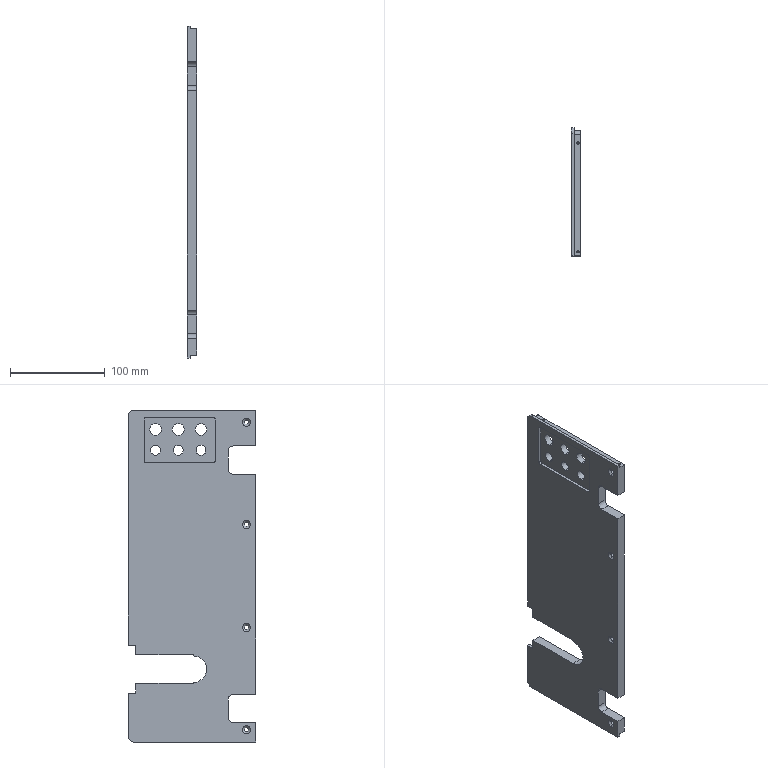Part | SolidWorks | features Cut 47, HoleWzd 41, MoveFace 39, ICE 28, Fillet 19, DelFace 17, MirrorPattern 3, SweepCut 2, Extrusion 1 | 1 solid | 111 faces | box 10 x 135 x 351 mm | volume 402993 mm3 | cylinder 51 | plane 34 | cone 26 | commonest cylinder face diameters 2.5 x18 4.5 x8 10.5 x6 12.5 x6 4 x4 10 x4